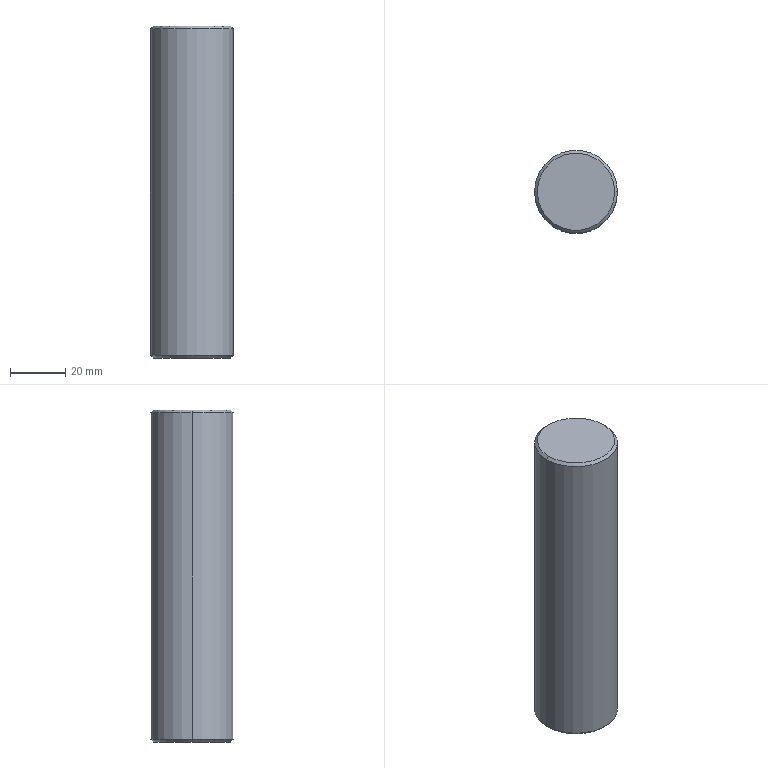Part | SolidWorks | 1 solid | 8 faces | box 30 x 30 x 120 mm | volume 84731 mm3 | cone 4 | cylinder 2 | plane 2 | commonest cylinder face diameters 30 x2
STEP:
#1=CARTESIAN_POINT('',(14.,0.,60.));
#2=VERTEX_POINT('',#1);
#3=CARTESIAN_POINT('',(-14.,0.,60.));
#4=VERTEX_POINT('',#3);
#5=CARTESIAN_POINT('',(0.,0.,60.));
#6=DIRECTION('',(0.,0.,1.));
#7=DIRECTION('',(1.,0.,0.));
#8=AXIS2_PLACEMENT_3D('',#5,#6,#7);
#9=CIRCLE('',#8,14.);
#10=EDGE_CURVE('',#2,#4,#9,.T.);
#11=ORIENTED_EDGE('',*,*,#10,.F.);
#12=CARTESIAN_POINT('',(15.,0.,59.));
#13=VERTEX_POINT('',#12);
#14=CARTESIAN_POINT('',(14.,0.,60.));
#15=DIRECTION('',(0.7071,0.,-0.7071));
#16=VECTOR('',#15,1000.);
#17=LINE('',#14,#16);
#18=EDGE_CURVE('',#2,#13,#17,.T.);
#19=ORIENTED_EDGE('',*,*,#18,.T.);
#20=CARTESIAN_POINT('',(-15.,0.,59.));
#21=VERTEX_POINT('',#20);
#22=CARTESIAN_POINT('',(0.,0.,59.));
#23=DIRECTION('',(0.,0.,-1.));
#24=DIRECTION('',(1.,0.,0.));
#25=AXIS2_PLACEMENT_3D('',#22,#23,#24);
#26=CIRCLE('',#25,15.);
#27=EDGE_CURVE('',#21,#13,#26,.T.);
#28=ORIENTED_EDGE('',*,*,#27,.F.);
#29=CARTESIAN_POINT('',(-14.,0.,60.));
#30=DIRECTION('',(-0.7071,0.,-0.7071));
#31=VECTOR('',#30,1000.);
#32=LINE('',#29,#31);
#33=EDGE_CURVE('',#4,#21,#32,.T.);
#34=ORIENTED_EDGE('',*,*,#33,.F.);
#35=EDGE_LOOP('',(#11,#19,#28,#34));
#36=FACE_OUTER_BOUND('',#35,.T.);
#37=CARTESIAN_POINT('',(0.,0.,60.));
#38=DIRECTION('',(0.,0.,-1.));
#39=DIRECTION('',(-1.,0.,0.));
#40=AXIS2_PLACEMENT_3D('',#37,#38,#39);
#41=CONICAL_SURFACE('',#40,14.,0.7854);
#42=ADVANCED_FACE('',(#36),#41,.T.);
#43=CARTESIAN_POINT('',(-14.,0.,-60.));
#44=VERTEX_POINT('',#43);
#45=CARTESIAN_POINT('',(14.,0.,-60.));
#46=VERTEX_POINT('',#45);
#47=CARTESIAN_POINT('',(0.,0.,-60.));
#48=DIRECTION('',(0.,0.,-1.));
#49=DIRECTION('',(1.,0.,0.));
#50=AXIS2_PLACEMENT_3D('',#47,#48,#49);
#51=CIRCLE('',#50,14.);
#52=EDGE_CURVE('',#44,#46,#51,.T.);
#53=ORIENTED_EDGE('',*,*,#52,.F.);
#54=CARTESIAN_POINT('',(-15.,0.,-59.));
#55=VERTEX_POINT('',#54);
#56=CARTESIAN_POINT('',(-15.,0.,-59.));
#57=DIRECTION('',(-0.7071,0.,0.7071));
#58=VECTOR('',#57,1000.);
#59=LINE('',#56,#58);
#60=EDGE_CURVE('',#44,#55,#59,.T.);
#61=ORIENTED_EDGE('',*,*,#60,.T.);
#62=CARTESIAN_POINT('',(15.,0.,-59.));
#63=VERTEX_POINT('',#62);
#64=CARTESIAN_POINT('',(0.,0.,-59.));
#65=DIRECTION('',(0.,0.,1.));
#66=DIRECTION('',(1.,0.,0.));
#67=AXIS2_PLACEMENT_3D('',#64,#65,#66);
#68=CIRCLE('',#67,15.);
#69=EDGE_CURVE('',#63,#55,#68,.T.);
#70=ORIENTED_EDGE('',*,*,#69,.F.);
#71=CARTESIAN_POINT('',(15.,0.,-59.));
#72=DIRECTION('',(0.7071,0.,0.7071));
#73=VECTOR('',#72,1000.);
#74=LINE('',#71,#73);
#75=EDGE_CURVE('',#46,#63,#74,.T.);
#76=ORIENTED_EDGE('',*,*,#75,.F.);
#77=EDGE_LOOP('',(#53,#61,#70,#76));
#78=FACE_OUTER_BOUND('',#77,.T.);
#79=CARTESIAN_POINT('',(0.,0.,-59.));
#80=DIRECTION('',(0.,0.,1.));
#81=DIRECTION('',(1.,0.,0.));
#82=AXIS2_PLACEMENT_3D('',#79,#80,#81);
#83=CONICAL_SURFACE('',#82,15.,0.7854);
#84=ADVANCED_FACE('',(#78),#83,.T.);
#85=ORIENTED_EDGE('',*,*,#27,.T.);
#86=CARTESIAN_POINT('',(15.,0.,60.));
#87=DIRECTION('',(0.,0.,-1.));
#88=VECTOR('',#87,1000.);
#89=LINE('',#86,#88);
#90=EDGE_CURVE('',#13,#63,#89,.T.);
#91=ORIENTED_EDGE('',*,*,#90,.T.);
#92=ORIENTED_EDGE('',*,*,#69,.T.);
#93=CARTESIAN_POINT('',(-15.,0.,60.));
#94=DIRECTION('',(0.,0.,-1.));
#95=VECTOR('',#94,1000.);
#96=LINE('',#93,#95);
#97=EDGE_CURVE('',#21,#55,#96,.T.);
#98=ORIENTED_EDGE('',*,*,#97,.F.);
#99=EDGE_LOOP('',(#85,#91,#92,#98));
#100=FACE_OUTER_BOUND('',#99,.T.);
#101=CARTESIAN_POINT('',(0.,0.,60.));
#102=DIRECTION('',(0.,0.,-1.));
#103=DIRECTION('',(-1.,0.,0.));
#104=AXIS2_PLACEMENT_3D('',#101,#102,#103);
#105=CYLINDRICAL_SURFACE('',#104,15.);
#106=ADVANCED_FACE('',(#100),#105,.T.);
#107=ORIENTED_EDGE('',*,*,#90,.F.);
#108=CARTESIAN_POINT('',(0.,0.,59.));
#109=DIRECTION('',(0.,0.,-1.));
#110=DIRECTION('',(1.,0.,0.));
#111=AXIS2_PLACEMENT_3D('',#108,#109,#110);
#112=CIRCLE('',#111,15.);
#113=EDGE_CURVE('',#13,#21,#112,.T.);
#114=ORIENTED_EDGE('',*,*,#113,.T.);
#115=ORIENTED_EDGE('',*,*,#97,.T.);
#116=CARTESIAN_POINT('',(0.,0.,-59.));
#117=DIRECTION('',(0.,0.,1.));
#118=DIRECTION('',(1.,0.,0.));
#119=AXIS2_PLACEMENT_3D('',#116,#117,#118);
#120=CIRCLE('',#119,15.);
#121=EDGE_CURVE('',#55,#63,#120,.T.);
#122=ORIENTED_EDGE('',*,*,#121,.T.);
#123=EDGE_LOOP('',(#107,#114,#115,#122));
#124=FACE_OUTER_BOUND('',#123,.T.);
#125=CARTESIAN_POINT('',(0.,0.,60.));
#126=DIRECTION('',(0.,0.,-1.));
#127=DIRECTION('',(-1.,0.,0.));
#128=AXIS2_PLACEMENT_3D('',#125,#126,#127);
#129=CYLINDRICAL_SURFACE('',#128,15.);
#130=ADVANCED_FACE('',(#124),#129,.T.);
#131=CARTESIAN_POINT('',(0.,0.,60.));
#132=DIRECTION('',(0.,0.,1.));
#133=DIRECTION('',(1.,0.,0.));
#134=AXIS2_PLACEMENT_3D('',#131,#132,#133);
#135=CIRCLE('',#134,14.);
#136=EDGE_CURVE('',#4,#2,#135,.T.);
#137=ORIENTED_EDGE('',*,*,#136,.T.);
#138=ORIENTED_EDGE('',*,*,#10,.T.);
#139=EDGE_LOOP('',(#137,#138));
#140=FACE_OUTER_BOUND('',#139,.T.);
#141=CARTESIAN_POINT('',(0.,0.,60.));
#142=DIRECTION('',(0.,0.,1.));
#143=DIRECTION('',(1.,0.,0.));
#144=AXIS2_PLACEMENT_3D('',#141,#142,#143);
#145=PLANE('',#144);
#146=ADVANCED_FACE('',(#140),#145,.T.);
#147=CARTESIAN_POINT('',(0.,0.,-60.));
#148=DIRECTION('',(0.,0.,-1.));
#149=DIRECTION('',(1.,0.,0.));
#150=AXIS2_PLACEMENT_3D('',#147,#148,#149);
#151=CIRCLE('',#150,14.);
#152=EDGE_CURVE('',#46,#44,#151,.T.);
#153=ORIENTED_EDGE('',*,*,#152,.T.);
#154=ORIENTED_EDGE('',*,*,#52,.T.);
#155=EDGE_LOOP('',(#153,#154));
#156=FACE_OUTER_BOUND('',#155,.T.);
#157=CARTESIAN_POINT('',(0.,0.,-60.));
#158=DIRECTION('',(0.,0.,1.));
#159=DIRECTION('',(1.,0.,0.));
#160=AXIS2_PLACEMENT_3D('',#157,#158,#159);
#161=PLANE('',#160);
#162=ADVANCED_FACE('',(#156),#161,.F.);
#163=ORIENTED_EDGE('',*,*,#60,.F.);
#164=ORIENTED_EDGE('',*,*,#152,.F.);
#165=ORIENTED_EDGE('',*,*,#75,.T.);
#166=ORIENTED_EDGE('',*,*,#121,.F.);
#167=EDGE_LOOP('',(#163,#164,#165,#166));
#168=FACE_OUTER_BOUND('',#167,.T.);
#169=CARTESIAN_POINT('',(0.,0.,-59.));
#170=DIRECTION('',(0.,0.,1.));
#171=DIRECTION('',(1.,0.,0.));
#172=AXIS2_PLACEMENT_3D('',#169,#170,#171);
#173=CONICAL_SURFACE('',#172,15.,0.7854);
#174=ADVANCED_FACE('',(#168),#173,.T.);
#175=ORIENTED_EDGE('',*,*,#18,.F.);
#176=ORIENTED_EDGE('',*,*,#136,.F.);
#177=ORIENTED_EDGE('',*,*,#33,.T.);
#178=ORIENTED_EDGE('',*,*,#113,.F.);
#179=EDGE_LOOP('',(#175,#176,#177,#178));
#180=FACE_OUTER_BOUND('',#179,.T.);
#181=CARTESIAN_POINT('',(0.,0.,60.));
#182=DIRECTION('',(0.,0.,-1.));
#183=DIRECTION('',(-1.,0.,0.));
#184=AXIS2_PLACEMENT_3D('',#181,#182,#183);
#185=CONICAL_SURFACE('',#184,14.,0.7854);
#186=ADVANCED_FACE('',(#180),#185,.T.);
#187=CLOSED_SHELL('',(#42,#84,#106,#130,#146,#162,#174,#186));
#188=MANIFOLD_SOLID_BREP('',#187);
#189=CARTESIAN_POINT('',(0.,0.,0.));
#190=DIRECTION('',(0.,0.,1.));
#191=DIRECTION('',(1.,0.,0.));
#192=AXIS2_PLACEMENT_3D('',#189,#190,#191);
#193=(LENGTH_UNIT()NAMED_UNIT(*)SI_UNIT(.MILLI.,.METRE.));
#194=UNCERTAINTY_MEASURE_WITH_UNIT(LENGTH_MEASURE(0.00001),#193,'','');
#195=(NAMED_UNIT(*)PLANE_ANGLE_UNIT()SI_UNIT($,.RADIAN.));
#196=(NAMED_UNIT(*)SI_UNIT($,.STERADIAN.)SOLID_ANGLE_UNIT());
#197=(GEOMETRIC_REPRESENTATION_CONTEXT(3)GLOBAL_UNCERTAINTY_ASSIGNED_CONTEXT((#194))GLOBAL_UNIT_ASSIGNED_CONTEXT((#193,#195,#196))REPRESENTATION_CONTEXT('',''));
#198=ADVANCED_BREP_SHAPE_REPRESENTATION('',(#188,#192),#197);